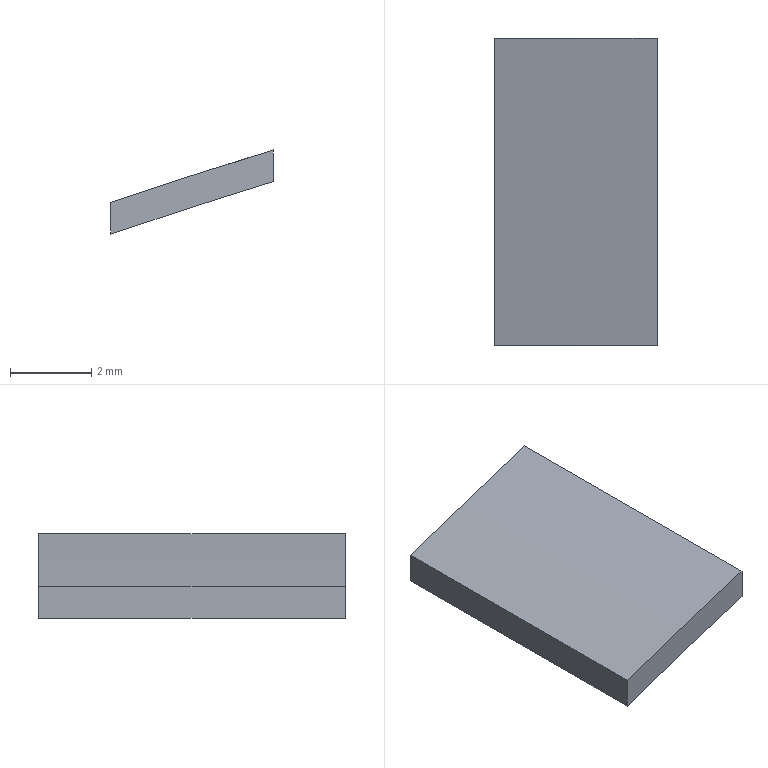Part | NX | features solid 2 | 1 solid | 6 faces | box 4 x 7.555 x 2.069 mm | volume 23.453 mm3 | plane 4 | spline 2
STEP:
#1=CARTESIAN_POINT('',(2.068,-12.879,17.304));
#2=VERTEX_POINT('',#1);
#3=CARTESIAN_POINT('',(-1.932,-12.879,16.011));
#4=VERTEX_POINT('',#3);
#5=CARTESIAN_POINT('',(2.068,-12.879,17.304));
#6=CARTESIAN_POINT('',(0.7288,-12.879,16.892));
#7=CARTESIAN_POINT('',(-0.6052,-12.879,16.461));
#8=CARTESIAN_POINT('',(-1.932,-12.879,16.011));
#9=B_SPLINE_CURVE_WITH_KNOTS('',3,(#5,#6,#7,#8),.UNSPECIFIED.,.F.,.F.,(4,4),(0.006318,0.01052),.UNSPECIFIED.);
#10=EDGE_CURVE('',#2,#4,#9,.T.);
#11=ORIENTED_EDGE('',*,*,#10,.T.);
#12=CARTESIAN_POINT('',(-1.932,-20.434,16.011));
#13=VERTEX_POINT('',#12);
#14=CARTESIAN_POINT('',(-1.932,-12.879,16.011));
#15=DIRECTION('',(0.,-1.,0.));
#16=VECTOR('',#15,1000.);
#17=LINE('',#14,#16);
#18=EDGE_CURVE('',#4,#13,#17,.T.);
#19=ORIENTED_EDGE('',*,*,#18,.T.);
#20=CARTESIAN_POINT('',(2.068,-20.434,17.304));
#21=VERTEX_POINT('',#20);
#22=CARTESIAN_POINT('',(-1.932,-20.434,16.011));
#23=CARTESIAN_POINT('',(-0.6059,-20.434,16.461));
#24=CARTESIAN_POINT('',(0.7292,-20.434,16.892));
#25=CARTESIAN_POINT('',(2.068,-20.434,17.304));
#26=B_SPLINE_CURVE_WITH_KNOTS('',3,(#22,#23,#24,#25),.UNSPECIFIED.,.F.,.F.,(4,4),(0.02434,0.02853),.UNSPECIFIED.);
#27=EDGE_CURVE('',#13,#21,#26,.T.);
#28=ORIENTED_EDGE('',*,*,#27,.T.);
#29=CARTESIAN_POINT('',(2.068,-16.657,17.304));
#30=DIRECTION('',(0.,-1.,0.));
#31=VECTOR('',#30,1000.);
#32=LINE('',#29,#31);
#33=EDGE_CURVE('',#21,#2,#32,.F.);
#34=ORIENTED_EDGE('',*,*,#33,.T.);
#35=EDGE_LOOP('',(#11,#19,#28,#34));
#36=FACE_BOUND('',#35,.T.);
#37=CARTESIAN_POINT('',(-1.932,-12.879,16.011));
#38=CARTESIAN_POINT('',(-1.932,-20.434,16.011));
#39=CARTESIAN_POINT('',(-0.604,-12.879,16.462));
#40=CARTESIAN_POINT('',(-0.604,-20.434,16.462));
#41=CARTESIAN_POINT('',(0.7294,-12.879,16.892));
#42=CARTESIAN_POINT('',(0.7294,-20.434,16.892));
#43=CARTESIAN_POINT('',(2.068,-12.879,17.304));
#44=CARTESIAN_POINT('',(2.068,-20.434,17.304));
#45=B_SPLINE_SURFACE_WITH_KNOTS('',3,1,((#37,#38),(#39,#40),(#41,#42),(#43,#44)),.SURF_OF_LINEAR_EXTRUSION.,.F.,.F.,.F.,(4,4),(2,2),(0.6832,0.7067),(0.,1.),.PIECEWISE_BEZIER_KNOTS.);
#46=ADVANCED_FACE('',(#36),#45,.F.);
#47=CARTESIAN_POINT('',(2.068,-12.879,16.528));
#48=VERTEX_POINT('',#47);
#49=CARTESIAN_POINT('',(2.068,-12.879,11.067));
#50=DIRECTION('',(0.,0.,1.));
#51=VECTOR('',#50,1000.);
#52=LINE('',#49,#51);
#53=EDGE_CURVE('',#48,#2,#52,.T.);
#54=ORIENTED_EDGE('',*,*,#53,.F.);
#55=CARTESIAN_POINT('',(-1.932,-12.879,15.234));
#56=VERTEX_POINT('',#55);
#57=CARTESIAN_POINT('',(-1.932,-12.879,15.234));
#58=CARTESIAN_POINT('',(-0.6049,-12.879,15.685));
#59=CARTESIAN_POINT('',(0.7285,-12.879,16.116));
#60=CARTESIAN_POINT('',(2.068,-12.879,16.528));
#61=B_SPLINE_CURVE_WITH_KNOTS('',3,(#57,#58,#59,#60),.UNSPECIFIED.,.F.,.F.,(4,4),(0.,0.004204),.UNSPECIFIED.);
#62=EDGE_CURVE('',#56,#48,#61,.T.);
#63=ORIENTED_EDGE('',*,*,#62,.F.);
#64=CARTESIAN_POINT('',(-1.932,-12.879,11.067));
#65=DIRECTION('',(0.,0.,1.));
#66=VECTOR('',#65,1000.);
#67=LINE('',#64,#66);
#68=EDGE_CURVE('',#56,#4,#67,.T.);
#69=ORIENTED_EDGE('',*,*,#68,.T.);
#70=ORIENTED_EDGE('',*,*,#10,.F.);
#71=EDGE_LOOP('',(#54,#63,#69,#70));
#72=FACE_BOUND('',#71,.T.);
#73=CARTESIAN_POINT('',(0.06794,-12.879,11.067));
#74=DIRECTION('',(0.,1.,0.));
#75=DIRECTION('',(0.,0.,-1.));
#76=AXIS2_PLACEMENT_3D('',#73,#74,#75);
#77=PLANE('',#76);
#78=ADVANCED_FACE('',(#72),#77,.T.);
#79=ORIENTED_EDGE('',*,*,#68,.F.);
#80=CARTESIAN_POINT('',(-1.932,-20.434,15.234));
#81=VERTEX_POINT('',#80);
#82=CARTESIAN_POINT('',(-1.932,-16.657,15.234));
#83=DIRECTION('',(0.,-1.,0.));
#84=VECTOR('',#83,1000.);
#85=LINE('',#82,#84);
#86=EDGE_CURVE('',#81,#56,#85,.F.);
#87=ORIENTED_EDGE('',*,*,#86,.F.);
#88=CARTESIAN_POINT('',(-1.932,-20.434,-70.255));
#89=DIRECTION('',(0.,0.,-1.));
#90=VECTOR('',#89,1000.);
#91=LINE('',#88,#90);
#92=EDGE_CURVE('',#81,#13,#91,.F.);
#93=ORIENTED_EDGE('',*,*,#92,.T.);
#94=ORIENTED_EDGE('',*,*,#18,.F.);
#95=EDGE_LOOP('',(#79,#87,#93,#94));
#96=FACE_BOUND('',#95,.T.);
#97=CARTESIAN_POINT('',(-1.932,-17.407,11.067));
#98=DIRECTION('',(-1.,0.,0.));
#99=DIRECTION('',(0.,0.,1.));
#100=AXIS2_PLACEMENT_3D('',#97,#98,#99);
#101=PLANE('',#100);
#102=ADVANCED_FACE('',(#96),#101,.T.);
#103=ORIENTED_EDGE('',*,*,#92,.F.);
#104=CARTESIAN_POINT('',(2.068,-20.434,16.528));
#105=VERTEX_POINT('',#104);
#106=CARTESIAN_POINT('',(2.068,-20.434,16.528));
#107=CARTESIAN_POINT('',(0.7285,-20.434,16.116));
#108=CARTESIAN_POINT('',(-0.6049,-20.434,15.685));
#109=CARTESIAN_POINT('',(-1.932,-20.434,15.234));
#110=B_SPLINE_CURVE_WITH_KNOTS('',3,(#106,#107,#108,#109),.UNSPECIFIED.,.F.,.F.,(4,4),(0.,0.004204),.UNSPECIFIED.);
#111=EDGE_CURVE('',#105,#81,#110,.T.);
#112=ORIENTED_EDGE('',*,*,#111,.F.);
#113=CARTESIAN_POINT('',(2.068,-20.434,11.067));
#114=DIRECTION('',(0.,0.,-1.));
#115=VECTOR('',#114,1000.);
#116=LINE('',#113,#115);
#117=EDGE_CURVE('',#105,#21,#116,.F.);
#118=ORIENTED_EDGE('',*,*,#117,.T.);
#119=ORIENTED_EDGE('',*,*,#27,.F.);
#120=EDGE_LOOP('',(#103,#112,#118,#119));
#121=FACE_BOUND('',#120,.T.);
#122=CARTESIAN_POINT('',(15.469,-20.434,-70.255));
#123=DIRECTION('',(0.,1.,0.));
#124=DIRECTION('',(-1.,0.,0.));
#125=AXIS2_PLACEMENT_3D('',#122,#123,#124);
#126=PLANE('',#125);
#127=ADVANCED_FACE('',(#121),#126,.F.);
#128=CARTESIAN_POINT('',(2.068,-16.657,16.528));
#129=DIRECTION('',(0.,-1.,0.));
#130=VECTOR('',#129,1000.);
#131=LINE('',#128,#130);
#132=EDGE_CURVE('',#48,#105,#131,.T.);
#133=ORIENTED_EDGE('',*,*,#132,.T.);
#134=ORIENTED_EDGE('',*,*,#111,.T.);
#135=ORIENTED_EDGE('',*,*,#86,.T.);
#136=ORIENTED_EDGE('',*,*,#62,.T.);
#137=EDGE_LOOP('',(#133,#134,#135,#136));
#138=FACE_BOUND('',#137,.T.);
#139=CARTESIAN_POINT('',(-1.932,-12.879,15.234));
#140=CARTESIAN_POINT('',(-1.932,-20.434,15.234));
#141=CARTESIAN_POINT('',(-0.6044,-12.879,15.685));
#142=CARTESIAN_POINT('',(-0.6044,-20.434,15.685));
#143=CARTESIAN_POINT('',(0.7291,-12.879,16.116));
#144=CARTESIAN_POINT('',(0.7291,-20.434,16.116));
#145=CARTESIAN_POINT('',(2.068,-12.879,16.528));
#146=CARTESIAN_POINT('',(2.068,-20.434,16.528));
#147=B_SPLINE_SURFACE_WITH_KNOTS('',3,1,((#139,#140),(#141,#142),(#143,#144),(#145,#146)),.SURF_OF_LINEAR_EXTRUSION.,.F.,.F.,.F.,(4,4),(2,2),(0.6828,0.7065),(0.,1.),.PIECEWISE_BEZIER_KNOTS.);
#148=ADVANCED_FACE('',(#138),#147,.T.);
#149=ORIENTED_EDGE('',*,*,#132,.F.);
#150=ORIENTED_EDGE('',*,*,#53,.T.);
#151=ORIENTED_EDGE('',*,*,#33,.F.);
#152=ORIENTED_EDGE('',*,*,#117,.F.);
#153=EDGE_LOOP('',(#149,#150,#151,#152));
#154=FACE_BOUND('',#153,.T.);
#155=CARTESIAN_POINT('',(2.068,-17.407,11.067));
#156=DIRECTION('',(1.,0.,0.));
#157=DIRECTION('',(0.,0.,-1.));
#158=AXIS2_PLACEMENT_3D('',#155,#156,#157);
#159=PLANE('',#158);
#160=ADVANCED_FACE('',(#154),#159,.T.);
#161=CLOSED_SHELL('',(#46,#78,#102,#127,#148,#160));
#162=MANIFOLD_SOLID_BREP('',#161);
#163=(LENGTH_UNIT()NAMED_UNIT(*)SI_UNIT(.MILLI.,.METRE.));
#164=UNCERTAINTY_MEASURE_WITH_UNIT(LENGTH_MEASURE(0.0508),#163,'','');
#165=(NAMED_UNIT(*)PLANE_ANGLE_UNIT()SI_UNIT($,.RADIAN.));
#166=(NAMED_UNIT(*)SI_UNIT($,.STERADIAN.)SOLID_ANGLE_UNIT());
#167=(GEOMETRIC_REPRESENTATION_CONTEXT(3)GLOBAL_UNCERTAINTY_ASSIGNED_CONTEXT((#164))GLOBAL_UNIT_ASSIGNED_CONTEXT((#163,#165,#166))REPRESENTATION_CONTEXT('',''));
#168=ADVANCED_BREP_SHAPE_REPRESENTATION('',(#162),#167);